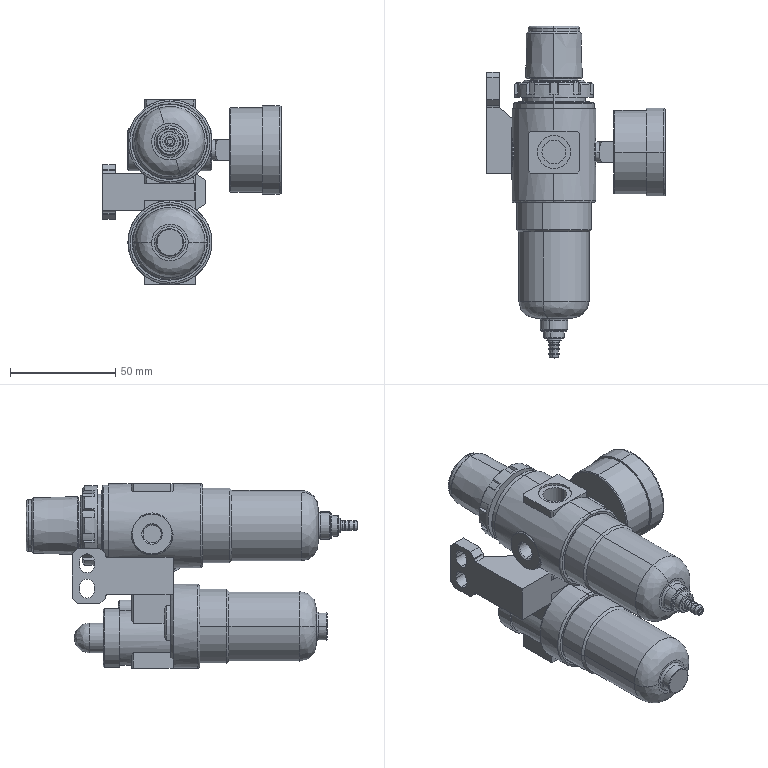Part | SolidWorks | 8 solids | 418 faces | box 85 x 158 x 88 mm | volume 192242 mm3 | plane 176 | cylinder 140 | cone 71 | spline 23 | torus 8 | commonest cylinder face diameters 35.2 x11 5 x8 7 x8 11.445 x8 13 x8 15.788 x8